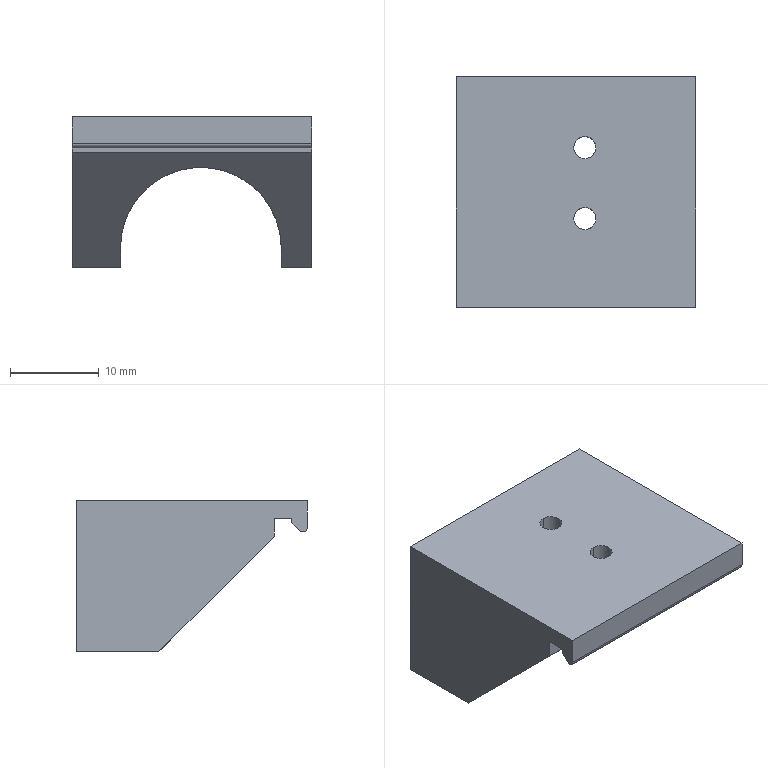NC program | NX | posted with a generic post | part box 27 x 26 x 17 mm
Lines 20452 to 21610 of 22937:
(ZLEVEL_PROFILE_1 , TOOL : D2R0.5)
N40854 T05 M6
N40856 G54
N40858 G17 G0 G90 X-8.739 Y2.619 S9500 M3
N40860 G43 Z30. H5
N40862 Z2.943
N40864 G94 G1 Z-0.057 F1000.
N40866 X-8.912 Y2.88
N40868 G3 X-9.091 Y2.97 R0.2
N40870 G1 X-9.146 Y2.966 F2500.
N40872 X-14.475 Y2.967
N40874 Y2.938 Z-0.085
N40876 Y2.91 Z-0.113
N40878 X-9.146
N40880 X-9.089 Y2.913
N40882 Y2.881 Z-0.141
N40884 X-9.088 Y2.857 Z-0.17
N40886 X-9.146 Y2.853
N40888 X-13.5
N40890 X-14.476 Y2.854
N40892 Y2.825 Z-0.198
N40894 Y2.797 Z-0.226
N40896 X-13.5
N40898 X-9.146
N40900 X-9.087 Y2.8
N40902 Y2.768 Z-0.255
N40904 X-9.086 Y2.743 Z-0.283
N40906 X-9.146 Y2.74
N40908 X-13.5
N40910 X-14.477 Y2.741
N40912 Y2.712 Z-0.311
N40914 Y2.684 Z-0.339
N40916 X-13.5 Y2.683
N40918 X-9.146
N40920 X-9.085 Y2.687
N40922 X-9.084 Y2.655 Z-0.368
N40924 Y2.63 Z-0.396
N40926 X-9.146 Y2.627
N40928 X-13.5
N40930 X-14.477 Y2.628
N40932 X-14.478 Y2.599 Z-0.424
N40934 Y2.571 Z-0.453
N40936 X-13.5 Y2.57
N40938 X-9.146
N40940 X-9.083 Y2.574
N40942 X-9.082 Y2.542 Z-0.481
N40944 Y2.517 Z-0.509
N40946 X-9.146 Y2.514
N40948 X-13.5
N40950 X-14.478
N40952 X-14.479 Y2.485 Z-0.537
N40954 Y2.458 Z-0.566
N40956 X-13.5 Y2.457
N40958 X-9.146
N40960 X-9.081 Y2.461
N40962 X-9.08 Y2.429 Z-0.594
N40964 X-9.079 Y2.404 Z-0.622
N40966 X-9.146 Y2.401
N40968 X-13.5
N40970 X-14.479
N40972 Y2.372 Z-0.651
N40974 X-14.48 Y2.345 Z-0.679
N40976 X-13.5 Y2.344
N40978 X-9.146
N40980 X-9.078 Y2.348
N40982 Y2.316 Z-0.707
N40984 X-9.077 Y2.291 Z-0.735
N40986 X-9.146 Y2.288
N40988 X-13.5
N40990 X-14.48
N40992 Y2.259 Z-0.764
N40994 X-14.481 Y2.231 Z-0.792
N40996 X-13.5
N40998 X-9.146
N41000 X-9.076 Y2.234
N41002 Y2.203 Z-0.82
N41004 X-9.075 Y2.178 Z-0.849
N41006 X-9.146 Y2.174
N41008 X-13.5
N41010 X-14.481 Y2.175
N41012 Y2.146 Z-0.877
N41014 Y2.118 Z-0.905
N41016 X-13.5
N41018 X-9.146
N41020 X-9.074 Y2.121
N41022 X-9.073 Y2.09 Z-0.933
N41024 Y2.065 Z-0.962
N41026 X-9.146 Y2.061
N41028 X-13.5
N41030 X-14.482 Y2.062
N41032 Y2.033 Z-0.99
N41034 Y2.005 Z-1.018
N41036 X-13.5
N41038 X-9.146
N41040 X-9.072 Y2.008
N41042 X-9.071 Y1.976 Z-1.047
N41044 Y1.951 Z-1.075
N41046 X-9.146 Y1.948
N41048 X-13.5
N41050 X-14.483 Y1.949
N41052 Y1.92 Z-1.103
N41054 Y1.892 Z-1.131
N41056 X-13.5
N41058 X-9.146
N41060 X-9.07 Y1.895
N41062 X-9.069 Y1.863 Z-1.16
N41064 X-9.068 Y1.838 Z-1.188
N41066 X-9.146 Y1.835
N41068 X-13.5
N41070 X-14.484
N41072 Y1.807 Z-1.216
N41074 Y1.779 Z-1.245
N41076 X-13.5 Y1.778
N41078 X-9.146
N41080 X-9.067 Y1.782
N41082 X-9.066 Y1.75 Z-1.273
N41084 Y1.725 Z-1.301
N41086 X-9.146 Y1.722
N41088 X-13.5
N41090 X-14.485
N41092 Y1.694 Z-1.329
N41094 Y1.666 Z-1.358
N41096 X-13.5 Y1.665
N41098 X-9.146
N41100 X-9.065 Y1.669
N41102 X-9.064 Y1.637 Z-1.386
N41104 X-9.063 Y1.612 Z-1.414
N41106 X-9.146 Y1.609
N41108 X-13.5
N41110 X-14.485
N41112 X-14.486 Y1.58 Z-1.442
N41114 Y1.553 Z-1.471
N41116 X-13.5 Y1.552
N41118 X-9.146
N41120 X-9.062 Y1.555
N41122 X-9.061 Y1.524 Z-1.499
N41124 Y1.499 Z-1.527
N41126 X-9.146 Y1.496
N41128 X-13.5
N41130 X-14.486
N41132 Y1.467 Z-1.556
N41134 X-14.487 Y1.439 Z-1.584
N41136 X-13.5
N41138 X-9.146
N41140 X-9.059 Y1.442
N41142 Y1.411 Z-1.612
N41144 X-9.058 Y1.386 Z-1.64
N41146 X-9.146 Y1.382
N41148 X-13.5
N41150 X-14.487 Y1.383
N41152 Y1.354 Z-1.669
N41154 Y1.326 Z-1.697
N41156 X-13.5
N41158 X-9.146
N41160 X-9.057 Y1.329
N41162 X-9.056 Y1.298 Z-1.725
N41164 X-9.055 Y1.272 Z-1.754
N41166 X-9.146 Y1.269
N41168 X-13.5
N41170 X-14.488 Y1.27
N41172 Y1.241 Z-1.782
N41174 Y1.213 Z-1.81
N41176 X-13.5
N41178 X-9.146
N41180 X-9.054 Y1.216
N41182 X-9.053 Y1.184 Z-1.838
N41184 Y1.159 Z-1.867
N41186 X-9.146 Y1.156
N41188 X-13.5
N41190 X-14.488
N41192 Y1.128 Z-1.895
N41194 X-14.489 Y1.1 Z-1.923
N41196 X-13.5
N41198 X-9.146
N41200 X-9.051 Y1.103
N41202 Y1.071 Z-1.952
N41204 X-9.05 Y1.046 Z-1.98
N41206 X-9.146 Y1.043
N41208 X-13.5
N41210 X-14.489
N41212 Y1.015 Z-2.008
N41214 Y0.987 Z-2.036
N41216 X-13.5 Y0.986
N41218 X-9.146
N41220 X-9.048 Y0.989
N41222 Y0.958 Z-2.065
N41224 X-9.047 Y0.933 Z-2.093
N41226 X-9.146 Y0.93
N41228 X-13.5
N41230 X-14.49
N41232 Y0.902 Z-2.121
N41234 Y0.874 Z-2.15
N41236 X-13.5 Y0.873
N41238 X-9.146
N41240 X-9.046 Y0.876
N41242 X-9.045 Y0.845 Z-2.178
N41244 X-9.044 Y0.82 Z-2.206
N41246 X-9.146 Y0.817
N41248 X-13.5
N41250 X-14.49
N41252 Y0.788 Z-2.234
N41254 X-14.491 Y0.76 Z-2.263
N41256 X-13.5
N41258 X-9.146
N41260 X-9.043 Y0.763
N41262 X-9.042 Y0.732 Z-2.291
N41264 X-9.041 Y0.706 Z-2.319
N41266 X-9.146 Y0.704
N41268 X-13.5
N41270 X-14.491
N41272 Y0.675 Z-2.348
N41274 Y0.647 Z-2.376
N41276 X-13.5
N41278 X-9.146
N41280 X-9.039 Y0.65
N41282 X-9.038 Y0.619 Z-2.404
N41284 X-9.037 Y0.593 Z-2.432
N41286 X-10.068 Y0.59
N41288 X-13.5
N41290 X-14.492 Y0.591
N41292 Y0.562 Z-2.461
N41294 Y0.534 Z-2.489
N41296 X-13.5
N41298 X-9.146
N41300 X-9.035 Y0.536
N41302 X-9.033 Y0.506 Z-2.517
N41304 X-9.032 Y0.48 Z-2.546
N41306 X-9.146 Y0.477
N41308 X-13.5
N41310 X-14.492 Y0.478
N41312 Y0.449 Z-2.574
N41314 X-14.493 Y0.421 Z-2.602
N41316 X-13.5
N41318 X-9.146
N41320 X-9.03 Y0.423
N41322 X-9.028 Y0.392 Z-2.63
N41324 X-9.027 Y0.366 Z-2.659
N41326 X-9.146 Y0.364
N41328 X-13.5
N41330 X-14.493
N41332 Y0.336 Z-2.687
N41334 Y0.308 Z-2.715
N41336 X-13.5
N41338 X-9.146
N41340 X-9.025 Y0.31
N41342 X-9.023 Y0.279 Z-2.744
N41344 X-9.021 Y0.253 Z-2.772
N41346 X-9.146 Y0.251
N41348 X-13.5
N41350 X-14.493
N41352 X-14.494 Y0.223 Z-2.8
N41354 Y0.195 Z-2.828
N41356 X-13.5 Y0.194
N41358 X-9.146
N41360 X-9.017 Y0.196
N41362 X-9.014 Y0.166 Z-2.857
N41364 X-9.013 Y0.14 Z-2.885
N41366 X-9.146 Y0.138
N41368 X-13.5
N41370 X-14.494
N41372 Y0.11 Z-2.913
N41374 Y0.082 Z-2.942
N41376 X-13.5 Y0.081
N41378 X-9.146
N41380 X-9.008 Y0.083
N41382 X-9.006 Y0.053 Z-2.97
N41384 X-9.004 Y0.026 Z-2.998
N41386 X-10.044 Y0.025
N41388 X-13.5
N41390 X-14.494
N41392 Y-0.004 Z-3.026
N41394 Y-0.032 Z-3.055
N41396 X-13.5
N41398 X-10.04
N41400 X-9. Y-0.031
N41402 X-8.997 Y-0.06 Z-3.083
N41404 X-8.995 Y-0.087 Z-3.111
N41406 X-10.036 Y-0.088
N41408 X-13.5
N41410 X-14.494
N41412 Y-0.117 Z-3.14
N41414 X-14.495 Y-0.145 Z-3.168
N41416 X-13.5
N41418 X-10.032
N41420 X-8.989 Y-0.144
N41422 X-8.986 Y-0.173 Z-3.196
N41424 X-8.983 Y-0.201 Z-3.224
N41426 X-10.027 Y-0.202
N41428 X-13.5
N41430 X-14.495 Y-0.201
N41432 Y-0.23 Z-3.253
N41434 Y-0.258 Z-3.281
N41436 X-13.5
N41438 X-10.02
N41440 X-8.976
N41442 X-8.973 Y-0.286 Z-3.309
N41444 X-8.97 Y-0.314 Z-3.338
N41446 X-10.013 Y-0.315
N41448 X-13.5
N41450 X-14.495 Y-0.314
N41452 Y-0.343 Z-3.366
N41454 Y-0.371 Z-3.394
N41456 X-13.5
N41458 X-10.007
N41460 X-8.964
N41462 X-8.96 Y-0.4 Z-3.422
N41464 X-8.957 Y-0.428 Z-3.451
N41466 X-10.
N41468 X-13.5
N41470 X-14.495
N41472 Y-0.456 Z-3.479
N41474 X-14.496 Y-0.484 Z-3.507
N41476 X-13.5
N41478 X-9.994
N41480 X-8.95
N41482 X-8.946 Y-0.513 Z-3.536
N41484 X-8.942 Y-0.54 Z-3.564
N41486 X-9.987 Y-0.541
N41488 X-13.5
N41490 X-14.496
N41492 Y-0.569 Z-3.592
N41494 Y-0.597 Z-3.62
N41496 X-13.5
N41498 X-8.947
N41500 X-8.933 Y-0.596
N41502 X-8.928 Y-0.626 Z-3.649
N41504 X-8.924 Y-0.652 Z-3.677
N41506 X-8.947 Y-0.654
N41508 X-13.5
N41510 X-14.496
N41512 Y-0.682 Z-3.705
N41514 Y-0.71 Z-3.734
N41516 X-13.5 Y-0.711
N41518 X-8.947
N41520 X-8.915 Y-0.708
N41522 X-8.909 Y-0.739 Z-3.762
N41524 X-8.905 Y-0.764 Z-3.79
N41526 X-8.947 Y-0.767
N41528 X-13.5
N41530 X-14.497
N41532 Y-0.795 Z-3.818
N41534 Y-0.824 Z-3.847
N41536 X-13.5
N41538 X-8.947
N41540 X-8.896 Y-0.82
N41542 X-8.891 Y-0.852 Z-3.875
N41544 X-8.887 Y-0.877 Z-3.903
N41546 X-8.947 Y-0.88
N41548 X-13.5
N41550 X-14.497
N41552 Y-0.909 Z-3.932
N41554 Y-0.937 Z-3.96
N41556 X-13.5
N41558 X-8.947
N41560 X-8.875 Y-0.933
N41562 X-8.868 Y-0.965 Z-3.988
N41564 X-8.863 Y-0.99 Z-4.016
N41566 X-8.947 Y-0.993
N41568 X-13.5
N41570 X-14.497
N41572 Y-1.022 Z-4.045
N41574 Y-1.05 Z-4.073
N41576 X-13.5
N41578 X-8.947
N41580 X-8.851 Y-1.047
N41582 X-8.845 Y-1.078 Z-4.101
N41584 X-8.84 Y-1.104 Z-4.13
N41586 X-8.947 Y-1.107
N41588 X-13.5
N41590 X-14.498 Y-1.106
N41592 Y-1.135 Z-4.158
N41594 Y-1.163 Z-4.186
N41596 X-13.5
N41598 X-8.947
N41600 X-8.828 Y-1.161
N41602 X-8.821 Y-1.191 Z-4.214
N41604 X-8.816 Y-1.218 Z-4.243
N41606 X-8.947 Y-1.22
N41608 X-13.5
N41610 X-14.498
N41612 Y-1.248 Z-4.271
N41614 Y-1.276 Z-4.299
N41616 X-13.5
N41618 X-9.855
N41620 X-8.804 Y-1.275
N41622 X-8.796 Y-1.305 Z-4.327
N41624 X-8.789 Y-1.332 Z-4.356
N41626 X-9.843 Y-1.333
N41628 X-13.5
N41630 X-14.498
N41632 Y-1.361 Z-4.384
N41634 Y-1.389 Z-4.412
N41636 X-13.5
N41638 X-9.831
N41640 X-8.775
N41642 X-8.767 Y-1.418 Z-4.441
N41644 X-8.76 Y-1.446 Z-4.469
N41646 X-9.817
N41648 X-13.5
N41650 X-14.498
N41652 Y-1.474 Z-4.497
N41654 Y-1.502 Z-4.525
N41656 X-13.5 Y-1.503
N41658 X-9.802
N41660 X-8.745 Y-1.502
N41662 X-8.737 Y-1.531 Z-4.554
N41664 X-8.73 Y-1.557 Z-4.582
N41666 X-8.748 Y-1.559
N41668 X-13.5
N41670 X-14.498
N41672 Y-1.587 Z-4.61
N41674 Y-1.616 Z-4.639
N41676 X-13.5
N41678 X-8.748
N41680 X-8.715 Y-1.613
N41682 X-8.707 Y-1.644 Z-4.667
N41684 X-8.701 Y-1.669 Z-4.695
N41686 X-8.748 Y-1.672
N41688 X-13.5
N41690 X-14.498
N41692 Y-1.701 Z-4.723
N41694 Y-1.729 Z-4.752
N41696 X-13.5
N41698 X-8.748
N41700 X-8.683 Y-1.725
N41702 X-8.666 Y-1.782 Z-4.808
N41704 X-8.748 Y-1.785
N41706 X-13.5
N41708 X-14.498
N41710 Y-1.814 Z-4.837
N41712 Y-1.842 Z-4.865
N41714 X-13.5
N41716 X-8.748
N41718 X-8.648 Y-1.839
N41720 X-8.63 Y-1.896 Z-4.921
N41722 X-8.748 Y-1.899
N41724 X-13.5
N41726 X-14.499 Y-1.898
N41728 Y-1.927 Z-4.95
N41730 Y-1.955 Z-4.978
N41732 X-13.5
N41734 X-8.748
N41736 X-8.612 Y-1.953
N41738 X-8.594 Y-2.01 Z-5.035
N41740 X-9.66 Y-2.012
N41742 X-13.5
N41744 X-14.499
N41746 Y-2.04 Z-5.063
N41748 Y-2.068 Z-5.091
N41750 X-13.5
N41752 X-9.642
N41754 X-8.576
N41756 X-8.556 Y-2.125 Z-5.148
N41758 X-9.625
N41760 X-13.5
N41762 X-14.499
N41764 Y-2.153 Z-5.176
N41766 Y-2.181 Z-5.204
N41768 X-13.5
N41770 X-8.549
N41772 X-8.536 Y-2.18
N41774 X-8.515 Y-2.235 Z-5.261
N41776 X-8.549 Y-2.238
N41778 X-13.5
N41780 X-14.499
N41782 Y-2.266 Z-5.289
N41784 Y-2.294 Z-5.317
N41786 X-13.5 Y-2.295
N41788 X-8.549
N41790 X-8.494 Y-2.291
N41792 X-8.473 Y-2.348 Z-5.374
N41794 X-8.549 Y-2.351
N41796 X-13.5
N41798 X-14.499
N41800 Y-2.379 Z-5.402
N41802 Y-2.408 Z-5.431
N41804 X-13.5
N41806 X-8.549
N41808 X-8.451 Y-2.404
N41810 X-8.43 Y-2.462 Z-5.487
N41812 X-8.549 Y-2.464
N41814 X-13.5
N41816 X-14.499
N41818 Y-2.493 Z-5.515
N41820 Y-2.521 Z-5.544
N41822 X-13.5
N41824 X-8.549
N41826 X-8.407 Y-2.519
N41828 X-8.383 Y-2.576 Z-5.6
N41830 X-9.466 Y-2.577
N41832 X-13.5
N41834 X-14.499
N41836 Y-2.606 Z-5.629
N41838 Y-2.634 Z-5.657
N41840 X-13.5
N41842 X-9.443
N41844 X-8.36
N41846 X-8.336 Y-2.689 Z-5.713
N41848 X-8.351 Y-2.691
N41850 X-13.5
N41852 X-14.499 Y-2.69
N41854 Y-2.719 Z-5.742
N41856 Y-2.747 Z-5.77
N41858 X-13.5
N41860 X-8.351
N41862 X-8.311 Y-2.744
N41864 X-8.286 Y-2.8 Z-5.827
N41866 X-8.351 Y-2.804
N41868 X-13.5
N41870 X-14.499
N41872 Y-2.832 Z-5.855
N41874 Y-2.86 Z-5.883
N41876 X-13.5
N41878 X-8.351
N41880 X-8.261 Y-2.857
N41882 X-8.235 Y-2.914 Z-5.94
N41884 X-8.351 Y-2.917
N41886 X-13.5
N41888 X-14.499
N41890 Y-2.945 Z-5.968
N41892 Y-2.973 Z-5.996
N41894 X-13.5
N41896 X-8.351
N41898 X-8.208 Y-2.971
N41900 X-8.181 Y-3.029 Z-6.053
N41902 X-9.277 Y-3.03
N41904 X-13.5
N41906 X-14.499
N41908 Y-3.058 Z-6.081
N41910 Y-3.086 Z-6.109
N41912 X-13.5 Y-3.087
N41914 X-9.251
N41916 X-8.155 Y-3.086
N41918 X-8.126 Y-3.141 Z-6.166
N41920 X-8.152 Y-3.143
N41922 X-13.5
N41924 X-14.499
N41926 Y-3.171 Z-6.194
N41928 Y-3.2 Z-6.223
N41930 X-13.5
N41932 X-8.152
N41934 X-8.097 Y-3.196
N41936 X-8.067 Y-3.253 Z-6.279
N41938 X-8.152 Y-3.256
N41940 X-13.5
N41942 X-14.499
N41944 Y-3.285 Z-6.307
N41946 Y-3.313 Z-6.336
N41948 X-13.5
N41950 X-8.152
N41952 X-8.038 Y-3.31
N41954 X-8.008 Y-3.367 Z-6.392
N41956 X-8.152 Y-3.369
N41958 X-13.5
N41960 X-14.499
N41962 Y-3.398 Z-6.421
N41964 Y-3.426 Z-6.449
N41966 X-13.5
N41968 X-9.088
N41970 X-7.978 Y-3.425
N41972 X-7.947 Y-3.482 Z-6.505
N41974 X-9.058
N41976 X-13.5
N41978 X-14.499
N41980 Y-3.511 Z-6.534
N41982 Y-3.539 Z-6.562
N41984 X-13.5
N41986 X-7.953
N41988 X-7.914 Y-3.536
N41990 X-7.881 Y-3.592 Z-6.619
N41992 X-7.953 Y-3.596
N41994 X-13.5
N41996 X-14.499
N41998 Y-3.624 Z-6.647
N42000 Y-3.652 Z-6.675
N42002 X-13.5
N42004 X-7.953
N42006 X-7.848 Y-3.649
N42008 X-7.814 Y-3.707 Z-6.732
N42010 X-7.953 Y-3.709
N42012 X-13.5
N42014 X-14.499
N42016 Y-3.737 Z-6.76
N42018 Y-3.765 Z-6.788
N42020 X-13.5
N42022 X-8.907
N42024 X-7.781 Y-3.764
N42026 X-7.747 Y-3.821 Z-6.845
N42028 X-8.874 Y-3.822
N42030 X-13.5
N42032 X-14.499
N42034 Y-3.85 Z-6.873
N42036 Y-3.878 Z-6.901
N42038 X-13.5
N42040 X-7.754
N42042 X-7.71 Y-3.877
N42044 X-7.673 Y-3.931 Z-6.958
N42046 X-7.754 Y-3.935
N42048 X-13.5
N42050 X-14.499
N42052 Y-3.963 Z-6.986
N42054 Y-3.991 Z-7.015
N42056 X-13.5 Y-3.992
N42058 X-7.754
N42060 X-7.636 Y-3.988
N42062 X-7.599 Y-4.047 Z-7.071
N42064 X-7.754 Y-4.048
N42066 X-13.5
N42068 X-14.499
N42070 Y-4.076 Z-7.099
N42072 Y-4.105 Z-7.128
N42074 X-13.5
N42076 X-8.707
N42078 X-7.562
N42080 X-7.523 Y-4.158 Z-7.184
N42082 X-7.555 Y-4.161
N42084 X-13.5
N42086 X-14.499
N42088 Y-4.19 Z-7.212
N42090 Y-4.218 Z-7.241
N42092 X-13.5
N42094 X-7.555
N42096 X-7.482 Y-4.214
N42098 X-7.442 Y-4.273 Z-7.297
N42100 X-8.597 Y-4.274
N42102 X-13.5
N42104 X-14.499
N42106 Y-4.303 Z-7.326
N42108 Y-4.331 Z-7.354
N42110 X-13.5
N42112 X-7.555
N42114 X-7.401 Y-4.329
N42116 X-7.36 Y-4.387 Z-7.41
N42118 X-8.523 Y-4.388
N42120 X-13.5
N42122 X-14.499 Y-4.387
N42124 Y-4.416 Z-7.439
N42126 Y-4.444 Z-7.467
N42128 X-13.5
N42130 X-7.356
N42132 X-7.318 Y-4.441
N42134 X-7.275 Y-4.497 Z-7.524
N42136 X-7.356 Y-4.501
N42138 X-13.5
N42140 X-14.499
N42142 Y-4.529 Z-7.552
N42144 Y-4.557 Z-7.58
N42146 X-13.5
N42148 X-7.356
N42150 X-7.23 Y-4.554
N42152 X-7.185 Y-4.612 Z-7.637
N42154 X-7.356 Y-4.614
N42156 X-13.5
N42158 X-14.499
N42160 Y-4.642 Z-7.665
N42162 Y-4.67 Z-7.693
N42164 X-13.5
N42166 X-7.158
N42168 X-7.141 Y-4.669
N42170 X-7.093 Y-4.723 Z-7.75
N42172 X-7.158 Y-4.727
N42174 X-13.5
N42176 X-14.499
N42178 Y-4.755 Z-7.778
N42180 Y-4.783 Z-7.806
N42182 X-13.5 Y-4.784
N42184 X-7.158
N42186 X-7.046 Y-4.779
N42188 X-6.998 Y-4.838 Z-7.863
N42190 X-7.158 Y-4.84
N42192 X-13.5
N42194 X-14.499
N42196 Y-4.868 Z-7.891
N42198 Y-4.897 Z-7.92
N42200 X-13.5
N42202 X-8.153
N42204 X-6.949 Y-4.896
N42206 X-6.899 Y-4.949 Z-7.976
N42208 X-6.959 Y-4.953
N42210 X-13.5
N42212 X-14.499
N42214 Y-4.982 Z-8.004
N42216 Y-5.01 Z-8.033
N42218 X-13.5
N42220 X-6.959
N42222 X-6.849 Y-5.006
N42224 X-6.799 Y-5.066 Z-8.089
N42226 X-8.019
N42228 X-13.5
N42230 X-14.499
N42232 Y-5.095 Z-8.118
N42234 Y-5.123 Z-8.146
N42236 X-13.5
N42238 X-6.76
N42240 X-6.745 Y-5.122
N42242 X-6.691 Y-5.175 Z-8.202
N42244 X-6.76 Y-5.18
N42246 X-13.5
N42248 X-14.499 Y-5.179
N42250 Y-5.208 Z-8.231
N42252 Y-5.236 Z-8.259
N42254 X-13.5
N42256 X-6.76
N42258 X-6.637 Y-5.233
N42260 X-6.583 Y-5.292 Z-8.316
N42262 X-7.826 Y-5.293
N42264 X-13.5
N42266 X-14.499
N42268 Y-5.321 Z-8.344
N42270 X-14.498 Y-5.349 Z-8.372
N42272 X-13.5
N42274 X-6.561
N42276 X-6.526 Y-5.346
N42278 X-6.467 Y-5.401 Z-8.429
N42280 X-6.561 Y-5.406
N42282 X-13.5
N42284 X-14.498
N42286 Y-5.434 Z-8.457
N42288 Y-5.462 Z-8.485
N42290 X-13.5
N42292 X-7.676
N42294 X-6.407 Y-5.461
N42296 X-6.347 Y-5.517 Z-8.542
N42298 X-6.362 Y-5.519
N42300 X-13.5
N42302 X-14.498
N42304 Y-5.547 Z-8.57
N42306 Y-5.575 Z-8.598
N42308 X-13.5 Y-5.576
N42310 X-6.362
N42312 X-6.285 Y-5.571
N42314 X-6.222 Y-5.629 Z-8.655
N42316 X-6.362 Y-5.632
N42318 X-13.5
N42320 X-14.498
N42322 Y-5.66 Z-8.683
N42324 Y-5.689 Z-8.712
N42326 X-13.5
N42328 X-7.46
N42330 X-6.159 Y-5.688
N42332 X-6.093 Y-5.741 Z-8.768
N42334 X-6.164 Y-5.745
N42336 X-13.5
N42338 X-14.498
N42340 Y-5.774 Z-8.796
N42342 Y-5.802 Z-8.825
N42344 X-13.5
N42346 X-6.164
N42348 X-6.026 Y-5.798
N42350 X-5.96 Y-5.858 Z-8.881
N42352 X-7.286
N42354 X-13.5
N42356 X-14.498
N42358 Y-5.887 Z-8.91
N42360 Y-5.915 Z-8.938
N42362 X-13.5
N42364 X-5.965
N42366 X-5.889 Y-5.911
N42368 X-5.817 Y-5.969 Z-8.994
N42370 X-5.965 Y-5.972
N42372 X-13.5
N42374 X-14.498 Y-5.971
N42376 Y-6. Z-9.023
N42378 Y-6.028 Z-9.051
N42380 X-13.5
N42382 X-5.766
N42384 X-5.745 Y-6.026
N42386 X-5.671 Y-6.082 Z-9.108
N42388 X-5.766 Y-6.085
N42390 X-13.5
N42392 X-14.497 Y-6.084
N42394 Y-6.113 Z-9.136
N42396 Y-6.141 Z-9.164
N42398 X-13.5
N42400 X-6.978
N42402 X-5.592 Y-6.14
N42404 X-5.514 Y-6.194 Z-9.221
N42406 X-5.567 Y-6.198
N42408 X-13.5
N42410 X-14.497
N42412 Y-6.226 Z-9.249
N42414 Y-6.254 Z-9.277
N42416 X-13.5
N42418 X-5.567
N42420 X-5.435 Y-6.252
N42422 X-5.393 Y-6.283 Z-9.306
N42424 X-5.352 Y-6.309 Z-9.334
N42426 X-5.368 Y-6.311
N42428 X-13.5
N42430 X-14.497
N42432 Y-6.339 Z-9.362
N42434 Y-6.367 Z-9.39
N42436 X-13.5
N42438 X-5.368
N42440 X-5.265 Y-6.363
N42442 X-5.221 Y-6.396 Z-9.419
N42444 X-5.178 Y-6.423 Z-9.447
N42446 X-6.639 Y-6.424
N42448 X-13.5
N42450 X-14.497
N42452 Y-6.452 Z-9.475
N42454 Y-6.48 Z-9.504
N42456 X-13.5 Y-6.481
N42458 X-5.169
N42460 X-5.089 Y-6.478
N42462 X-5.042 Y-6.509 Z-9.532
N42464 X-4.994 Y-6.536 Z-9.56
N42466 X-6.497 Y-6.537
N42468 X-13.5
N42470 X-14.496
N42472 Y-6.565 Z-9.588
N42474 Y-6.594 Z-9.617
N42476 X-13.5
N42478 X-4.971
N42480 X-4.899 Y-6.588
N42482 X-4.85 Y-6.622 Z-9.645
N42484 X-4.802 Y-6.648 Z-9.673
N42486 X-4.971 Y-6.65
N42488 X-13.5
N42490 X-14.496
N42492 Y-6.679 Z-9.702
N42494 Y-6.707 Z-9.73
N42496 X-13.5
N42498 X-4.772
N42500 X-4.699 Y-6.704
N42502 X-4.645 Y-6.735 Z-9.758
N42504 X-4.592 Y-6.762 Z-9.786
N42506 X-6.185 Y-6.763
N42508 X-13.5
N42510 X-14.496
N42512 Y-6.792 Z-9.815
N42514 Y-6.82 Z-9.843
N42516 X-13.5
N42518 X-4.573
N42520 X-4.482 Y-6.815
N42522 X-4.425 Y-6.848 Z-9.871
N42524 X-4.368 Y-6.876 Z-9.899
N42526 X-6.018 Y-6.877
N42528 X-13.5
N42530 X-14.495 Y-6.876
N42532 Y-6.905 Z-9.928
N42534 Y-6.933 Z-9.956
N42536 X-13.5
N42538 X-4.374
N42540 X-4.248 Y-6.93
N42542 X-4.186 Y-6.961 Z-9.984
N42544 X-4.124 Y-6.985 Z-10.013
N42546 X-4.175 Y-6.99
N42548 X-13.5
N42550 X-14.495
N42552 Y-7.018 Z-10.041
N42554 Y-7.046 Z-10.069
N42556 X-13.5
N42558 X-4.175
N42560 X-3.992 Y-7.045
N42562 X-3.924 Y-7.075 Z-10.097
N42564 X-3.857 Y-7.101 Z-10.126
N42566 X-3.976 Y-7.103
N42568 X-13.5
N42570 X-14.495
N42572 Y-7.131 Z-10.154
N42574 Y-7.159 Z-10.182
N42576 X-13.5
N42578 X-3.778
N42580 X-3.712 Y-7.156
N42582 X-3.634 Y-7.188 Z-10.211
N42584 X-3.556 Y-7.215 Z-10.239
N42586 X-5.467 Y-7.216
N42588 X-13.5
N42590 X-14.494
N42592 Y-7.244 Z-10.267
N42594 Y-7.272 Z-10.295
N42596 X-13.5 Y-7.273
N42598 X-5.366
N42600 X-3.397 Y-7.272
N42602 X-3.313 Y-7.301 Z-10.324
N42604 X-3.23 Y-7.327 Z-10.352
N42606 X-3.38 Y-7.329
N42608 X-13.5
N42610 X-14.494
N42612 Y-7.357 Z-10.38
N42614 Y-7.386 Z-10.409
N42616 X-13.5
N42618 X-3.181
N42620 X-3.056 Y-7.382
N42622 X-2.991 Y-7.405 Z-10.427
N42624 X-2.926 Y-7.423 Z-10.446
N42626 X-2.861 Y-7.44 Z-10.465
N42628 X-2.982 Y-7.442
N42630 X-13.5
N42632 X-14.494
N42634 Y-7.471 Z-10.493
N42636 X-14.493 Y-7.499 Z-10.522
N42638 X-13.5
N42640 X-4.923
N42642 X-2.632 Y-7.498
N42644 G2 X-2.459 Y-7.598 R0.2
N42646 G1 X-2.291 Y-7.888
N42648 Z-7.522
N42650 G0 Z30.
N42652 X14.795 Y2.612
N42654 Z2.943
N42656 G1 Z-0.057 F1000.
N42658 X14.648 Y2.867
N42660 G3 X14.475 Y2.967 R0.2
N42662 G1 X7.158 Y2.966 F2500.
N42664 X7.091 Y2.97
N42666 X7.09 Y2.938 Z-0.085
N42668 X7.089 Y2.913 Z-0.113
N42670 X7.158 Y2.91
N42672 X14.475
N42674 Y2.881 Z-0.141
N42676 X14.476 Y2.854 Z-0.17
N42678 X13.5 Y2.853
N42680 X7.158
N42682 X7.088 Y2.857
N42684 Y2.825 Z-0.198
N42686 X7.087 Y2.8 Z-0.226
N42688 X7.158 Y2.797
N42690 X13.5
N42692 X14.476
N42694 Y2.768 Z-0.255
N42696 X14.477 Y2.741 Z-0.283
N42698 X13.5 Y2.74
N42700 X7.158
N42702 X7.086 Y2.743
N42704 X7.085 Y2.712 Z-0.311
N42706 Y2.687 Z-0.339
N42708 X7.158 Y2.683
N42710 X13.5
N42712 X14.477 Y2.684
N42714 Y2.655 Z-0.368
N42716 Y2.628 Z-0.396
N42718 X13.5 Y2.627
N42720 X7.158
N42722 X7.084 Y2.63
N42724 X7.083 Y2.599 Z-0.424
N42726 Y2.574 Z-0.453
N42728 X7.158 Y2.57
N42730 X13.5
N42732 X14.478 Y2.571
N42734 Y2.542 Z-0.481
N42736 Y2.514 Z-0.509
N42738 X13.5
N42740 X7.158
N42742 X7.082 Y2.517
N42744 X7.081 Y2.485 Z-0.537
N42746 Y2.461 Z-0.566
N42748 X7.158 Y2.457
N42750 X13.5
N42752 X14.479 Y2.458
N42754 Y2.429 Z-0.594
N42756 Y2.401 Z-0.622
N42758 X13.5
N42760 X7.158
N42762 X7.079 Y2.404
N42764 Y2.372 Z-0.651
N42766 X7.078 Y2.347 Z-0.679
N42768 X7.158 Y2.344
N42770 X13.5
N42772 X14.48 Y2.345
N42774 Y2.316 Z-0.707
N42776 Y2.288 Z-0.735
N42778 X13.5
N42780 X7.158
N42782 X7.077 Y2.291
N42784 Y2.259 Z-0.764
N42786 X7.076 Y2.234 Z-0.792
N42788 X7.158 Y2.231
N42790 X13.5
N42792 X14.48
N42794 X14.481 Y2.203 Z-0.82
N42796 Y2.175 Z-0.849
N42798 X13.5 Y2.174
N42800 X7.158
N42802 X7.075 Y2.178
N42804 X7.074 Y2.146 Z-0.877
N42806 Y2.121 Z-0.905
N42808 X7.158 Y2.118
N42810 X13.5
N42812 X14.481
N42814 X14.482 Y2.09 Z-0.933
N42816 Y2.062 Z-0.962
N42818 X13.5 Y2.061
N42820 X7.158
N42822 X7.073 Y2.064
N42824 X7.072 Y2.033 Z-0.99
N42826 Y2.008 Z-1.018
N42828 X7.158 Y2.005
N42830 X13.5
N42832 X14.482
N42834 Y1.976 Z-1.047
N42836 X14.483 Y1.949 Z-1.075
N42838 X13.5 Y1.948
N42840 X7.158
N42842 X7.071 Y1.951
N42844 X7.07 Y1.92 Z-1.103
N42846 Y1.895 Z-1.131
N42848 X7.158 Y1.892
N42850 X13.5
N42852 X14.483
N42854 Y1.863 Z-1.16
N42856 X14.484 Y1.835 Z-1.188
N42858 X13.5
N42860 X7.158
N42862 X7.068 Y1.838
N42864 Y1.807 Z-1.216
N42866 X7.067 Y1.782 Z-1.245
N42868 X7.158 Y1.778
N42870 X13.5
N42872 X14.484 Y1.779
N42874 Y1.75 Z-1.273
N42876 Y1.722 Z-1.301
N42878 X13.5
N42880 X7.158
N42882 X7.066 Y1.725
N42884 X7.065 Y1.694 Z-1.329
N42886 Y1.668 Z-1.358
N42888 X7.158 Y1.665
N42890 X13.5
N42892 X14.485 Y1.666
N42894 Y1.637 Z-1.386
N42896 Y1.609 Z-1.414
N42898 X13.5
N42900 X7.158
N42902 X7.063 Y1.612
N42904 Y1.58 Z-1.442
N42906 X7.062 Y1.555 Z-1.471
N42908 X7.158 Y1.552
N42910 X13.5
N42912 X14.486 Y1.553
N42914 Y1.524 Z-1.499
N42916 Y1.496 Z-1.527
N42918 X13.5
N42920 X7.158
N42922 X7.061 Y1.499
N42924 X7.06 Y1.467 Z-1.556
N42926 X7.059 Y1.442 Z-1.584
N42928 X7.158 Y1.439
N42930 X13.5
N42932 X14.487
N42934 Y1.411 Z-1.612
N42936 Y1.383 Z-1.64
N42938 X13.5 Y1.382
N42940 X7.158
N42942 X7.058 Y1.385
N42944 X7.057 Y1.354 Z-1.669
N42946 Y1.329 Z-1.697
N42948 X7.158 Y1.326
N42950 X13.5
N42952 X14.487
N42954 Y1.298 Z-1.725
N42956 X14.488 Y1.27 Z-1.754
N42958 X13.5 Y1.269
N42960 X7.158
N42962 X7.055 Y1.272
N42964 Y1.241 Z-1.782
N42966 X7.054 Y1.215 Z-1.81
N42968 X7.158 Y1.213
N42970 X13.5
N42972 X14.488
N42974 Y1.184 Z-1.838
N42976 Y1.156 Z-1.867
N42978 X13.5
N42980 X7.158
N42982 X7.053 Y1.159
N42984 X7.052 Y1.128 Z-1.895
N42986 X7.051 Y1.102 Z-1.923
N42988 X7.158 Y1.1
N42990 X13.5
N42992 X14.489
N42994 Y1.071 Z-1.952
N42996 Y1.043 Z-1.98
N42998 X13.5
N43000 X7.158
N43002 X7.05 Y1.046
N43004 X7.049 Y1.015 Z-2.008
N43006 X7.048 Y0.989 Z-2.036
N43008 X7.158 Y0.986
N43010 X13.5
N43012 X14.489 Y0.987
N43014 Y0.958 Z-2.065
N43016 Y0.93 Z-2.093
N43018 X13.5
N43020 X7.158
N43022 X7.047 Y0.932
N43024 X7.046 Y0.902 Z-2.121
N43026 Y0.876 Z-2.15
N43028 X7.158 Y0.873
N43030 X13.5
N43032 X14.49 Y0.874
N43034 Y0.845 Z-2.178
N43036 Y0.817 Z-2.206
N43038 X13.5
N43040 X7.158
N43042 X7.044 Y0.819
N43044 Y0.788 Z-2.234
N43046 X7.043 Y0.763 Z-2.263
N43048 X7.158 Y0.76
N43050 X13.5
N43052 X14.49
N43054 X14.491 Y0.732 Z-2.291
N43056 Y0.704 Z-2.319
N43058 X13.5
N43060 X7.158
N43062 X7.041 Y0.706
N43064 X7.04 Y0.675 Z-2.348
N43066 X7.039 Y0.649 Z-2.376
N43068 X7.158 Y0.647
N43070 X13.5
N43072 X14.491
N43074 Y0.619 Z-2.404
N43076 Y0.591 Z-2.432
N43078 X13.5 Y0.59
N43080 X7.158
N43082 X7.037 Y0.593
N43084 X7.036 Y0.562 Z-2.461
N43086 X7.035 Y0.536 Z-2.489
N43088 X7.158 Y0.534
N43090 X13.5
N43092 X14.492
N43094 Y0.506 Z-2.517
N43096 Y0.478 Z-2.546
N43098 X13.5 Y0.477
N43100 X7.158
N43102 X7.032 Y0.479
N43104 X7.031 Y0.449 Z-2.574
N43106 X7.03 Y0.423 Z-2.602
N43108 X7.158 Y0.421
N43110 X13.5
N43112 X14.492
N43114 X14.493 Y0.392 Z-2.63
N43116 Y0.364 Z-2.659
N43118 X13.5
N43120 X7.158
N43122 X7.027 Y0.366
N43124 X7.026 Y0.336 Z-2.687
N43126 X7.025 Y0.309 Z-2.715
N43128 X7.158 Y0.308
N43130 X13.5
N43132 X14.493
N43134 Y0.279 Z-2.744
N43136 Y0.251 Z-2.772
N43138 X13.5
N43140 X7.158
N43142 X7.021 Y0.253
N43144 X7.019 Y0.223 Z-2.8
N43146 X7.017 Y0.196 Z-2.828
N43148 X8.056 Y0.194
N43150 X13.5
N43152 X14.494 Y0.195
N43154 Y0.166 Z-2.857
N43156 Y0.138 Z-2.885
N43158 X13.5
N43160 X8.052
N43162 X7.013 Y0.139
N43164 X7.01 Y0.11 Z-2.913